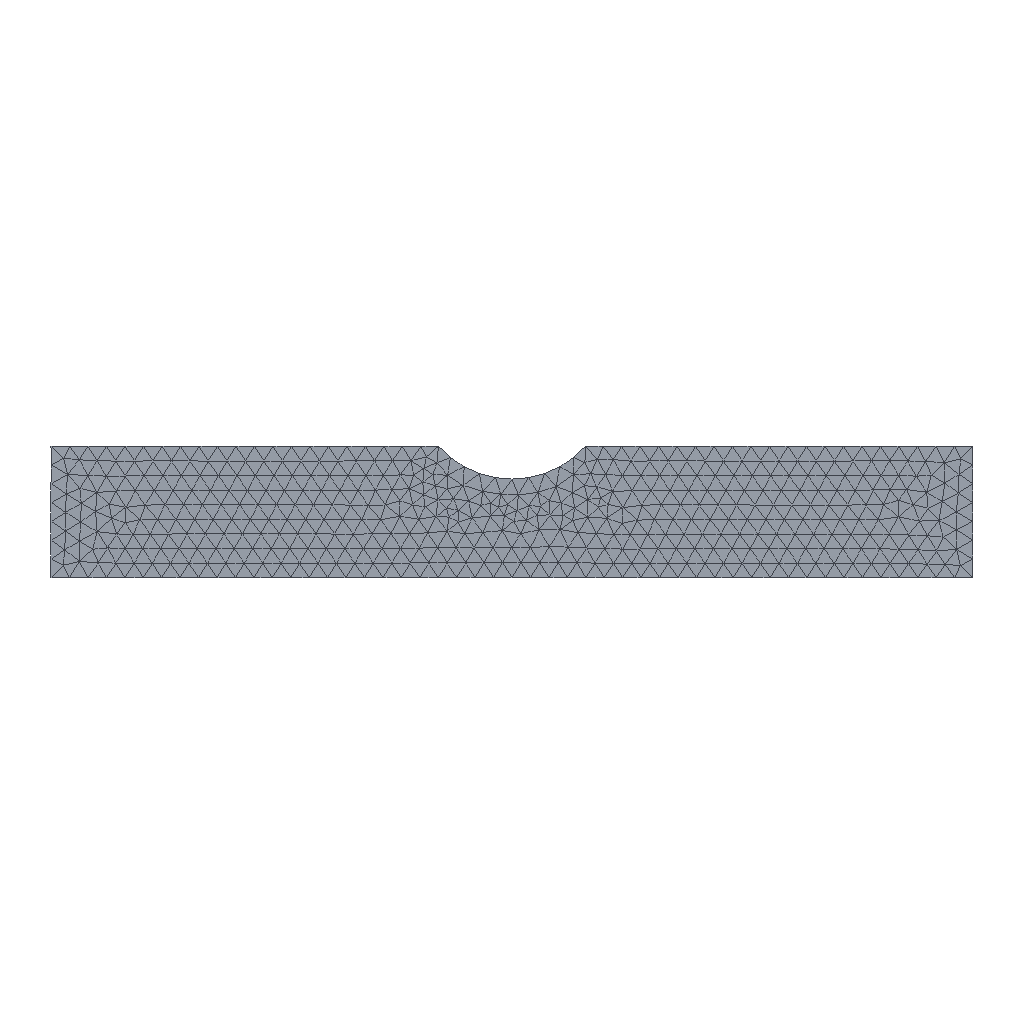Simulation study | comsol
Set-up summary:
category,name,step,type,value,unit,region
solver,comsol,,COMSOL Multiphysics 6.4 (Build: 293)
units,SI; geometry length unit m,,stated,COMSOL default unit system (SI)
analysis,Study 1,,Transient,space_dimension=2D
load_step,std1/time,std1/time,Transient,"type=Transient; times=range(0,1,10)"
mesh,nodes,,,519
mesh,elements,,,920
element_type,tri,,,920
element_type,edg,,,116
element_type,vtx,,,7
component,mod1,,2D,geometry=geom1; domains=1
physics,Electric Currents (ec),mod1,ConductiveMedia,V(V)
physics,Moving Mesh (ale),mod1,MovingMesh
parameter,K,,,1.0e-11[m^3/(A*s)]
bc,Current Conservation 1 (cucn1),mod1/ec,CurrentConservationSolid,sigma=10; rho0=0; Tref=293.15[K]; alpha=0; epsilonr=1; epsilonBis=0; epsilonPrim=1; delta=0; P=0 0 0; Dr=0 0 0; ConstitutiveRelationDE=RelativePermittivity; materialType=solid; ConstitutiveRelationJcE=ElectricalConductivity; HallCoef=0; sigma0=0; HallEffectMagneticFluxDensity=0 0 0; tanDelta=0; epsilonrS=1,,selection [1]
bc,Electric Insulation 1 (ein1),mod1/ec,ElectricInsulation,,,selection []
bc,Initial Values 1 (init1),mod1/ec,init,V=0,,selection [1]
bc,Continuity (dcont1),mod1/ec,Continuity,pairDisconnect=1; nitscheFormulation=skew; applyOn=dst; stabilizationTerm=automatic; stabilizationFactor=1; pairSelection=all; pairsList=0,,selection []
bc,Electric Insulation 2 (ein2),mod1/ec,ElectricInsulation,,,"selection [1, 5]"
bc,Ground 1 (gnd1),mod1/ec,Ground,V0=0,,selection [2]
bc,Electric Potential 1 (pot1),mod1/ec,ElectricPotential,V0=30,,"selection [3, 4, 6, 7]"
bc,Fixed Mesh 1 (fix1),mod1/ale,FixedMesh,,,selection []
bc,Prescribed Mesh Displacement 1 (disp1),mod1/ale,PrescribedMeshDisplacement,useDx=1 1; dx=0 0; weakConstraints=1,,selection [2]
bc,Free Deformation 1 (free1),mod1/ale,FreeDeformation,dxInit=0 0,,selection [1]
bc,Prescribed Mesh Velocity 1 (vel1),mod1/ale,PrescribedMeshVelocity,useVx=1 0; vx=0 0; weakConstraints=1,,"selection [1, 5]"
bc,Prescribed Mesh Velocity 2 (vel2),mod1/ale,PrescribedMeshVelocity,useVx=0 1; vx=0 -K*(-ec.nJ); weakConstraints=1,,"selection [3, 4, 6, 7]"
COMSOL model file for Java, long lists of numbers shortened:
/*
 * em_deck.java
 */

import com.comsol.model.*;
import com.comsol.model.util.*;

/** Model exported on Oct 28 2026, 10:37 by COMSOL 6.4.0.293. */
public class em_deck {

  public static Model run() {
    Model model = ModelUtil.create("Model");

    model.modelPath("");

    model.label("in.mph");

    model.param().set("K", "1.0e-11[m^3/(A*s)]", "Proportionality constant");

    model.component().create("mod1", false);

    model.component("mod1").geom().create("geom1", 2);

    model.component("mod1").label("Model 1");

    model.component("mod1").defineLocalCoord(false);

    model.component("mod1").curvedInterior(false);

    model.component("mod1").mesh().create("mesh1");

    model.component("mod1").geom("geom1").repairTolType("relative");
    model.component("mod1").geom("geom1").create("r1", "Rectangle");
    model.component("mod1").geom("geom1").feature("r1").set("size", new String[]{"2.8e-3", "0.4e-3"});
    model.component("mod1").geom("geom1").feature("r1").set("pos", new String[]{"-1.4e-3", "0e-3"});
    model.component("mod1").geom("geom1").create("c1", "Circle");
    model.component("mod1").geom("geom1").feature("c1").set("r", "0.3e-3");
    model.component("mod1").geom("geom1").feature("c1").set("pos", new String[]{"0", "0.6e-3"});
    model.component("mod1").geom("geom1").create("dif1", "Difference");
    model.component("mod1").geom("geom1").feature("dif1").selection("input").set("r1");
    model.component("mod1").geom("geom1").feature("dif1").selection("input2").set("c1");
    model.component("mod1").geom("geom1").feature("fin").set("repairtoltype", "relative");
    model.component("mod1").geom("geom1").run();

    model.component("mod1").coordSystem().create("sys2", "Boundary");

    model.component("mod1").physics().create("ec", "ConductiveMedia", "geom1");
    model.component("mod1").physics("ec").create("cucn1", "CurrentConservationSolid", 2);
    model.component("mod1").physics("ec").feature("cucn1").selection().all();
    model.component("mod1").physics("ec").feature("cucn1").featureInfo().create("information");
    model.component("mod1").physics("ec").create("ein2", "ElectricInsulation", 1);
    model.component("mod1").physics("ec").feature("ein2").selection().set(1, 5);
    model.component("mod1").physics("ec").create("gnd1", "Ground", 1);
    model.component("mod1").physics("ec").feature("gnd1").selection().set(2);
    model.component("mod1").physics("ec").create("pot1", "ElectricPotential", 1);
    model.component("mod1").physics("ec").feature("pot1").selection().set(3, 4, 6, 7);
    model.component("mod1").physics().create("ale", "MovingMesh", "geom1");
    model.component("mod1").physics("ale").create("free1", "FreeDeformation", 2);
    model.component("mod1").physics("ale").feature("free1").selection().set(1);
    model.component("mod1").physics("ale").create("vel1", "PrescribedMeshVelocity", 1);
    model.component("mod1").physics("ale").feature("vel1").selection().set(1, 5);
    model.component("mod1").physics("ale").create("vel2", "PrescribedMeshVelocity", 1);
    model.component("mod1").physics("ale").feature("vel2").selection().set(3, 4, 6, 7);

    model.component("mod1").mesh("mesh1").autoMeshSize(2);

    model.thermodynamics().label("Thermodynamics Package");

    model.component("mod1").view("view1").set("showlabels", true);
    model.component("mod1").view("view1").axis().set("xmin", -0.00154);
    model.component("mod1").view("view1").axis().set("xmax", 0.00154);
    model.component("mod1").view("view1").axis().set("ymin", -0.001642);
    model.component("mod1").view("view1").axis().set("ymax", 0.002117);

    model.component("mod1").coordSystem("sys2").label("Material Boundary System 2");
    model.component("mod1").coordSystem("sys2").set("frametype", "material");

    model.component("mod1").physics("ec").prop("ShapeProperty").set("frame", "material");
    model.component("mod1").physics("ec").prop("d").set("d", "2.8e-3");
    model.component("mod1").physics("ec").prop("PortSweepSettings").set("PortParamName", "PortName");
    model.component("mod1").physics("ec").prop("PortSweepSettings").set("zref", 50);
    model.component("mod1").physics("ec").feature("cucn1").set("sigma_mat", "userdef");
    model.component("mod1").physics("ec").feature("cucn1")
         .set("sigma", new int[][]{{10}, {0}, {0}, {0}, {10}, {0}, {0}, {0}, {10}});
    model.component("mod1").physics("ec").feature("cucn1").set("rho0", 0);
    model.component("mod1").physics("ec").feature("cucn1").set("Tref", "293.15[K]");
    model.component("mod1").physics("ec").feature("cucn1").set("epsilonr_mat", "userdef");
    model.component("mod1").physics("ec").feature("cucn1")
         .set("epsilonBis", new int[][]{{0}, {0}, {0}, {0}, {0}, {0}, {0}, {0}, {0}});
    model.component("mod1").physics("ec").feature("cucn1").set("minput_temperature_src", "userdef");
    model.component("mod1").physics("ec").feature("cucn1").set("minput_electricfield_src", "root.mod1.ec.EX");
    model.component("mod1").physics("ec").feature("cucn1").label("Current Conservation 1");
    model.component("mod1").physics("ec").feature("cucn1").featureInfo("information").label("Migrated Feature");
    model.component("mod1").physics("ec").feature("dcont1").set("pairDisconnect", true);
    model.component("mod1").physics("ec").feature("dcont1").label("Continuity");
    model.component("mod1").physics("ec").feature("pot1").set("V0", 30);
    model.component("mod1").physics("ale").prop("freeDeformationControlsBoundaries")
         .set("freeDeformationControlsBoundaries", 1);
    model.component("mod1").physics("ale").feature("disp1").set("weakConstraints", true);
    model.component("mod1").physics("ale").feature("vel1").set("useVx", new int[][]{{1}, {0}});
    model.component("mod1").physics("ale").feature("vel1").set("weakConstraints", true);
    model.component("mod1").physics("ale").feature("vel2").set("useVx", new int[][]{{0}, {1}});
    model.component("mod1").physics("ale").feature("vel2").set("vx", new String[][]{{"0"}, {"-K*(-ec.nJ)"}});
    model.component("mod1").physics("ale").feature("vel2").set("weakConstraints", true);
    model.component("mod1").physics("ale").feature("vel2").set("coordinateSystem", "sys1");

    model.study().create("std1");
    model.study("std1").create("time", "Transient");

    model.sol().create("sol1");
    model.sol("sol1").attach("std1");
    model.sol("sol1").create("st1", "StudyStep");
    model.sol("sol1").create("v1", "Variables");
    model.sol("sol1").create("t1", "Time");
    model.sol("sol1").feature("t1").create("fc1", "FullyCoupled");
    model.sol("sol1").feature("t1").feature().remove("fcDef");

    model.result().create("pg1", "PlotGroup2D");
    model.result("pg1").create("surf1", "Surface");
    model.result("pg1").feature("surf1").set("data", "dset1");
    model.result("pg1").feature("surf1").set("expr", "ec.normJ");

    model.study("std1").feature("time").set("tlist", "range(0,1,10)");

    model.sol("sol1").label("Solver 1");
    model.sol("sol1").feature("st1").label("Compile Equations: Time Dependent");
    model.sol("sol1").feature("v1").label("Dependent Variables 1.1");
    model.sol("sol1").feature("v1").set("clistctrl", new String[]{});
    model.sol("sol1").feature("v1").set("cname", new String[]{});
    model.sol("sol1").feature("v1").set("clist", new int[]{});
    model.sol("sol1").feature("t1").label("Time-Dependent Solver 1.1");
    model.sol("sol1").feature("t1").set("tlist", "range(0,1,10)");
    model.sol("sol1").feature("t1").set("atolglobalvaluemethod", "manual");
    model.sol("sol1").feature("t1").set("atolglobal", "0.001");
    model.sol("sol1").feature("t1").set("ewtrescale", false);
    model.sol("sol1").feature("t1")
         .set("atolvaluemethod", new String[]{"mod1_V", "manual", "mod1_spatial_disp", "manual", "mod1_spatial_disp_lm", "manual"});
    model.sol("sol1").feature("t1").set("initialstepbdf", "0.001");
    model.sol("sol1").feature("t1").set("bwinitstepfrac", "1.0");
    model.sol("sol1").feature("t1").feature("dDef").label("Direct 1");
    model.sol("sol1").feature("t1").feature("dDef").set("thresh", 0.1);
    model.sol("sol1").feature("t1").feature("dDef").set("ooc", false);
    model.sol("sol1").feature("t1").feature("dDef").set("rhob", 400);
    model.sol("sol1").feature("t1").feature("aDef").label("Advanced 1");
    model.sol("sol1").feature("t1").feature("fc1").label("Fully Coupled 1.1");
    model.sol("sol1").feature("t1").feature("fc1").set("probesel", "manual");

    model.study("std1").runNoGen();

    model.result().dataset("dset1").label("Solution 1");
    model.result("pg1").set("smooth", "internal");
    model.result("pg1").feature("surf1").set("colortable", "RainbowClassic");
    model.result("pg1").feature("surf1").set("smooth", "internal");
    model.result("pg1").feature("surf1").set("resolution", "normal");

    return model;
  }

  public static void main(String[] args) {
    run();
  }

}
Results summary:
result,max V = abs(mod1.V),dset1 (11 solution(s)),,30,V